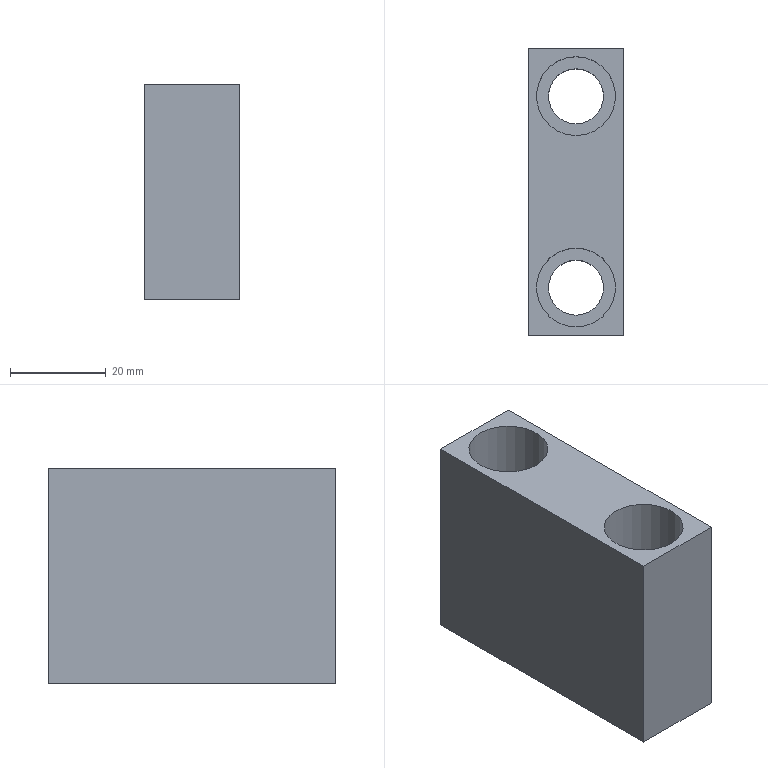Part | NX | features solid 2 | 1 solid | 12 faces | box 20 x 60 x 45 mm | volume 40254 mm3 | plane 8 | cylinder 4 | commonest cylinder face diameters 11.5 x2 16.5 x2
STEP:
#1=CARTESIAN_POINT('',(285.,200.,192.5));
#2=VERTEX_POINT('',#1);
#3=CARTESIAN_POINT('',(285.,200.,147.5));
#4=VERTEX_POINT('',#3);
#5=CARTESIAN_POINT('',(285.,200.,192.5));
#6=DIRECTION('',(0.,0.,-1.));
#7=VECTOR('',#6,1000.);
#8=LINE('',#5,#7);
#9=EDGE_CURVE('',#2,#4,#8,.T.);
#10=ORIENTED_EDGE('',*,*,#9,.F.);
#11=CARTESIAN_POINT('',(285.,140.,192.5));
#12=VERTEX_POINT('',#11);
#13=CARTESIAN_POINT('',(285.,200.,192.5));
#14=DIRECTION('',(0.,-1.,0.));
#15=VECTOR('',#14,1000.);
#16=LINE('',#13,#15);
#17=EDGE_CURVE('',#2,#12,#16,.T.);
#18=ORIENTED_EDGE('',*,*,#17,.T.);
#19=CARTESIAN_POINT('',(285.,140.,147.5));
#20=VERTEX_POINT('',#19);
#21=CARTESIAN_POINT('',(285.,140.,192.5));
#22=DIRECTION('',(0.,0.,-1.));
#23=VECTOR('',#22,1000.);
#24=LINE('',#21,#23);
#25=EDGE_CURVE('',#12,#20,#24,.T.);
#26=ORIENTED_EDGE('',*,*,#25,.T.);
#27=CARTESIAN_POINT('',(285.,200.,147.5));
#28=DIRECTION('',(0.,1.,0.));
#29=VECTOR('',#28,1000.);
#30=LINE('',#27,#29);
#31=EDGE_CURVE('',#4,#20,#30,.F.);
#32=ORIENTED_EDGE('',*,*,#31,.F.);
#33=EDGE_LOOP('',(#10,#18,#26,#32));
#34=FACE_BOUND('',#33,.T.);
#35=CARTESIAN_POINT('',(285.,200.,192.5));
#36=DIRECTION('',(1.,0.,0.));
#37=DIRECTION('',(0.,-1.,0.));
#38=AXIS2_PLACEMENT_3D('',#35,#36,#37);
#39=PLANE('',#38);
#40=ADVANCED_FACE('',(#34),#39,.T.);
#41=ORIENTED_EDGE('',*,*,#25,.F.);
#42=CARTESIAN_POINT('',(265.,140.,192.5));
#43=VERTEX_POINT('',#42);
#44=CARTESIAN_POINT('',(285.,140.,192.5));
#45=DIRECTION('',(-1.,0.,0.));
#46=VECTOR('',#45,1000.);
#47=LINE('',#44,#46);
#48=EDGE_CURVE('',#12,#43,#47,.T.);
#49=ORIENTED_EDGE('',*,*,#48,.T.);
#50=CARTESIAN_POINT('',(265.,140.,147.5));
#51=VERTEX_POINT('',#50);
#52=CARTESIAN_POINT('',(265.,140.,192.5));
#53=DIRECTION('',(0.,0.,-1.));
#54=VECTOR('',#53,1000.);
#55=LINE('',#52,#54);
#56=EDGE_CURVE('',#43,#51,#55,.T.);
#57=ORIENTED_EDGE('',*,*,#56,.T.);
#58=CARTESIAN_POINT('',(285.,140.,147.5));
#59=DIRECTION('',(1.,0.,0.));
#60=VECTOR('',#59,1000.);
#61=LINE('',#58,#60);
#62=EDGE_CURVE('',#20,#51,#61,.F.);
#63=ORIENTED_EDGE('',*,*,#62,.F.);
#64=EDGE_LOOP('',(#41,#49,#57,#63));
#65=FACE_BOUND('',#64,.T.);
#66=CARTESIAN_POINT('',(285.,140.,192.5));
#67=DIRECTION('',(0.,-1.,0.));
#68=DIRECTION('',(-1.,0.,0.));
#69=AXIS2_PLACEMENT_3D('',#66,#67,#68);
#70=PLANE('',#69);
#71=ADVANCED_FACE('',(#65),#70,.T.);
#72=ORIENTED_EDGE('',*,*,#56,.F.);
#73=CARTESIAN_POINT('',(265.,200.,192.5));
#74=VERTEX_POINT('',#73);
#75=CARTESIAN_POINT('',(265.,200.,192.5));
#76=DIRECTION('',(0.,-1.,0.));
#77=VECTOR('',#76,1000.);
#78=LINE('',#75,#77);
#79=EDGE_CURVE('',#74,#43,#78,.T.);
#80=ORIENTED_EDGE('',*,*,#79,.F.);
#81=CARTESIAN_POINT('',(265.,200.,147.5));
#82=VERTEX_POINT('',#81);
#83=CARTESIAN_POINT('',(265.,200.,192.5));
#84=DIRECTION('',(0.,0.,-1.));
#85=VECTOR('',#84,1000.);
#86=LINE('',#83,#85);
#87=EDGE_CURVE('',#74,#82,#86,.T.);
#88=ORIENTED_EDGE('',*,*,#87,.T.);
#89=CARTESIAN_POINT('',(265.,200.,147.5));
#90=DIRECTION('',(0.,1.,0.));
#91=VECTOR('',#90,1000.);
#92=LINE('',#89,#91);
#93=EDGE_CURVE('',#82,#51,#92,.F.);
#94=ORIENTED_EDGE('',*,*,#93,.T.);
#95=EDGE_LOOP('',(#72,#80,#88,#94));
#96=FACE_BOUND('',#95,.T.);
#97=CARTESIAN_POINT('',(265.,200.,192.5));
#98=DIRECTION('',(1.,0.,0.));
#99=DIRECTION('',(0.,-1.,0.));
#100=AXIS2_PLACEMENT_3D('',#97,#98,#99);
#101=PLANE('',#100);
#102=ADVANCED_FACE('',(#96),#101,.F.);
#103=CARTESIAN_POINT('',(285.,200.,192.5));
#104=DIRECTION('',(-1.,0.,0.));
#105=VECTOR('',#104,1000.);
#106=LINE('',#103,#105);
#107=EDGE_CURVE('',#2,#74,#106,.T.);
#108=ORIENTED_EDGE('',*,*,#107,.F.);
#109=ORIENTED_EDGE('',*,*,#9,.T.);
#110=CARTESIAN_POINT('',(285.,200.,147.5));
#111=DIRECTION('',(1.,0.,0.));
#112=VECTOR('',#111,1000.);
#113=LINE('',#110,#112);
#114=EDGE_CURVE('',#4,#82,#113,.F.);
#115=ORIENTED_EDGE('',*,*,#114,.T.);
#116=ORIENTED_EDGE('',*,*,#87,.F.);
#117=EDGE_LOOP('',(#108,#109,#115,#116));
#118=FACE_BOUND('',#117,.T.);
#119=CARTESIAN_POINT('',(285.,200.,192.5));
#120=DIRECTION('',(0.,-1.,0.));
#121=DIRECTION('',(-1.,0.,0.));
#122=AXIS2_PLACEMENT_3D('',#119,#120,#121);
#123=PLANE('',#122);
#124=ADVANCED_FACE('',(#118),#123,.F.);
#125=CARTESIAN_POINT('',(275.,195.75,147.5));
#126=VERTEX_POINT('',#125);
#127=CARTESIAN_POINT('',(275.,190.,147.5));
#128=DIRECTION('',(0.,0.,-1.));
#129=DIRECTION('',(0.,1.,0.));
#130=AXIS2_PLACEMENT_3D('',#127,#128,#129);
#131=CIRCLE('',#130,5.75);
#132=EDGE_CURVE('',#126,#126,#131,.T.);
#133=ORIENTED_EDGE('',*,*,#132,.F.);
#134=EDGE_LOOP('',(#133));
#135=FACE_BOUND('',#134,.T.);
#136=CARTESIAN_POINT('',(275.,155.75,147.5));
#137=VERTEX_POINT('',#136);
#138=CARTESIAN_POINT('',(275.,150.,147.5));
#139=DIRECTION('',(0.,0.,-1.));
#140=DIRECTION('',(0.,1.,0.));
#141=AXIS2_PLACEMENT_3D('',#138,#139,#140);
#142=CIRCLE('',#141,5.75);
#143=EDGE_CURVE('',#137,#137,#142,.T.);
#144=ORIENTED_EDGE('',*,*,#143,.F.);
#145=EDGE_LOOP('',(#144));
#146=FACE_BOUND('',#145,.T.);
#147=ORIENTED_EDGE('',*,*,#93,.F.);
#148=ORIENTED_EDGE('',*,*,#114,.F.);
#149=ORIENTED_EDGE('',*,*,#31,.T.);
#150=ORIENTED_EDGE('',*,*,#62,.T.);
#151=EDGE_LOOP('',(#147,#148,#149,#150));
#152=FACE_BOUND('',#151,.T.);
#153=CARTESIAN_POINT('',(285.,200.,147.5));
#154=DIRECTION('',(0.,0.,-1.));
#155=DIRECTION('',(0.,1.,0.));
#156=AXIS2_PLACEMENT_3D('',#153,#154,#155);
#157=PLANE('',#156);
#158=ADVANCED_FACE('',(#135,#146,#152),#157,.T.);
#159=CARTESIAN_POINT('',(275.,198.25,192.5));
#160=VERTEX_POINT('',#159);
#161=CARTESIAN_POINT('',(275.,190.,192.5));
#162=DIRECTION('',(0.,0.,-1.));
#163=DIRECTION('',(0.,1.,0.));
#164=AXIS2_PLACEMENT_3D('',#161,#162,#163);
#165=CIRCLE('',#164,8.25);
#166=EDGE_CURVE('',#160,#160,#165,.T.);
#167=ORIENTED_EDGE('',*,*,#166,.T.);
#168=EDGE_LOOP('',(#167));
#169=FACE_BOUND('',#168,.T.);
#170=CARTESIAN_POINT('',(275.,158.25,192.5));
#171=VERTEX_POINT('',#170);
#172=CARTESIAN_POINT('',(275.,150.,192.5));
#173=DIRECTION('',(0.,0.,-1.));
#174=DIRECTION('',(0.,1.,0.));
#175=AXIS2_PLACEMENT_3D('',#172,#173,#174);
#176=CIRCLE('',#175,8.25);
#177=EDGE_CURVE('',#171,#171,#176,.T.);
#178=ORIENTED_EDGE('',*,*,#177,.T.);
#179=EDGE_LOOP('',(#178));
#180=FACE_BOUND('',#179,.T.);
#181=ORIENTED_EDGE('',*,*,#79,.T.);
#182=ORIENTED_EDGE('',*,*,#48,.F.);
#183=ORIENTED_EDGE('',*,*,#17,.F.);
#184=ORIENTED_EDGE('',*,*,#107,.T.);
#185=EDGE_LOOP('',(#181,#182,#183,#184));
#186=FACE_BOUND('',#185,.T.);
#187=CARTESIAN_POINT('',(285.,200.,192.5));
#188=DIRECTION('',(0.,0.,-1.));
#189=DIRECTION('',(0.,1.,0.));
#190=AXIS2_PLACEMENT_3D('',#187,#188,#189);
#191=PLANE('',#190);
#192=ADVANCED_FACE('',(#169,#180,#186),#191,.F.);
#193=ORIENTED_EDGE('',*,*,#143,.T.);
#194=EDGE_LOOP('',(#193));
#195=FACE_BOUND('',#194,.T.);
#196=CARTESIAN_POINT('',(275.,155.75,172.5));
#197=VERTEX_POINT('',#196);
#198=CARTESIAN_POINT('',(275.,150.,172.5));
#199=DIRECTION('',(0.,0.,-1.));
#200=DIRECTION('',(0.,1.,0.));
#201=AXIS2_PLACEMENT_3D('',#198,#199,#200);
#202=CIRCLE('',#201,5.75);
#203=EDGE_CURVE('',#197,#197,#202,.T.);
#204=ORIENTED_EDGE('',*,*,#203,.F.);
#205=EDGE_LOOP('',(#204));
#206=FACE_BOUND('',#205,.T.);
#207=CARTESIAN_POINT('',(275.,150.,142.5));
#208=DIRECTION('',(0.,0.,-1.));
#209=DIRECTION('',(0.,1.,0.));
#210=AXIS2_PLACEMENT_3D('',#207,#208,#209);
#211=CYLINDRICAL_SURFACE('',#210,5.75);
#212=ADVANCED_FACE('',(#195,#206),#211,.F.);
#213=ORIENTED_EDGE('',*,*,#203,.T.);
#214=EDGE_LOOP('',(#213));
#215=FACE_BOUND('',#214,.T.);
#216=CARTESIAN_POINT('',(275.,158.25,172.5));
#217=VERTEX_POINT('',#216);
#218=CARTESIAN_POINT('',(275.,150.,172.5));
#219=DIRECTION('',(0.,0.,-1.));
#220=DIRECTION('',(0.,1.,0.));
#221=AXIS2_PLACEMENT_3D('',#218,#219,#220);
#222=CIRCLE('',#221,8.25);
#223=EDGE_CURVE('',#217,#217,#222,.T.);
#224=ORIENTED_EDGE('',*,*,#223,.F.);
#225=EDGE_LOOP('',(#224));
#226=FACE_BOUND('',#225,.T.);
#227=CARTESIAN_POINT('',(275.,150.,172.5));
#228=DIRECTION('',(0.,0.,-1.));
#229=DIRECTION('',(0.,1.,0.));
#230=AXIS2_PLACEMENT_3D('',#227,#228,#229);
#231=PLANE('',#230);
#232=ADVANCED_FACE('',(#215,#226),#231,.F.);
#233=ORIENTED_EDGE('',*,*,#223,.T.);
#234=EDGE_LOOP('',(#233));
#235=FACE_BOUND('',#234,.T.);
#236=ORIENTED_EDGE('',*,*,#177,.F.);
#237=EDGE_LOOP('',(#236));
#238=FACE_BOUND('',#237,.T.);
#239=CARTESIAN_POINT('',(275.,150.,192.5));
#240=DIRECTION('',(0.,0.,-1.));
#241=DIRECTION('',(0.,1.,0.));
#242=AXIS2_PLACEMENT_3D('',#239,#240,#241);
#243=CYLINDRICAL_SURFACE('',#242,8.25);
#244=ADVANCED_FACE('',(#235,#238),#243,.F.);
#245=ORIENTED_EDGE('',*,*,#132,.T.);
#246=EDGE_LOOP('',(#245));
#247=FACE_BOUND('',#246,.T.);
#248=CARTESIAN_POINT('',(275.,195.75,172.5));
#249=VERTEX_POINT('',#248);
#250=CARTESIAN_POINT('',(275.,190.,172.5));
#251=DIRECTION('',(0.,0.,-1.));
#252=DIRECTION('',(0.,1.,0.));
#253=AXIS2_PLACEMENT_3D('',#250,#251,#252);
#254=CIRCLE('',#253,5.75);
#255=EDGE_CURVE('',#249,#249,#254,.T.);
#256=ORIENTED_EDGE('',*,*,#255,.F.);
#257=EDGE_LOOP('',(#256));
#258=FACE_BOUND('',#257,.T.);
#259=CARTESIAN_POINT('',(275.,190.,142.5));
#260=DIRECTION('',(0.,0.,-1.));
#261=DIRECTION('',(0.,1.,0.));
#262=AXIS2_PLACEMENT_3D('',#259,#260,#261);
#263=CYLINDRICAL_SURFACE('',#262,5.75);
#264=ADVANCED_FACE('',(#247,#258),#263,.F.);
#265=ORIENTED_EDGE('',*,*,#255,.T.);
#266=EDGE_LOOP('',(#265));
#267=FACE_BOUND('',#266,.T.);
#268=CARTESIAN_POINT('',(275.,198.25,172.5));
#269=VERTEX_POINT('',#268);
#270=CARTESIAN_POINT('',(275.,190.,172.5));
#271=DIRECTION('',(0.,0.,-1.));
#272=DIRECTION('',(0.,1.,0.));
#273=AXIS2_PLACEMENT_3D('',#270,#271,#272);
#274=CIRCLE('',#273,8.25);
#275=EDGE_CURVE('',#269,#269,#274,.T.);
#276=ORIENTED_EDGE('',*,*,#275,.F.);
#277=EDGE_LOOP('',(#276));
#278=FACE_BOUND('',#277,.T.);
#279=CARTESIAN_POINT('',(275.,190.,172.5));
#280=DIRECTION('',(0.,0.,-1.));
#281=DIRECTION('',(0.,1.,0.));
#282=AXIS2_PLACEMENT_3D('',#279,#280,#281);
#283=PLANE('',#282);
#284=ADVANCED_FACE('',(#267,#278),#283,.F.);
#285=ORIENTED_EDGE('',*,*,#275,.T.);
#286=EDGE_LOOP('',(#285));
#287=FACE_BOUND('',#286,.T.);
#288=ORIENTED_EDGE('',*,*,#166,.F.);
#289=EDGE_LOOP('',(#288));
#290=FACE_BOUND('',#289,.T.);
#291=CARTESIAN_POINT('',(275.,190.,192.5));
#292=DIRECTION('',(0.,0.,-1.));
#293=DIRECTION('',(0.,1.,0.));
#294=AXIS2_PLACEMENT_3D('',#291,#292,#293);
#295=CYLINDRICAL_SURFACE('',#294,8.25);
#296=ADVANCED_FACE('',(#287,#290),#295,.F.);
#297=CLOSED_SHELL('',(#40,#71,#102,#124,#158,#192,#212,#232,#244,#264,#284,#296));
#298=MANIFOLD_SOLID_BREP('',#297);
#299=(LENGTH_UNIT()NAMED_UNIT(*)SI_UNIT(.MILLI.,.METRE.));
#300=UNCERTAINTY_MEASURE_WITH_UNIT(LENGTH_MEASURE(0.00001),#299,'','');
#301=(NAMED_UNIT(*)PLANE_ANGLE_UNIT()SI_UNIT($,.RADIAN.));
#302=(NAMED_UNIT(*)SI_UNIT($,.STERADIAN.)SOLID_ANGLE_UNIT());
#303=(GEOMETRIC_REPRESENTATION_CONTEXT(3)GLOBAL_UNCERTAINTY_ASSIGNED_CONTEXT((#300))GLOBAL_UNIT_ASSIGNED_CONTEXT((#299,#301,#302))REPRESENTATION_CONTEXT('',''));
#304=ADVANCED_BREP_SHAPE_REPRESENTATION('',(#298),#303);